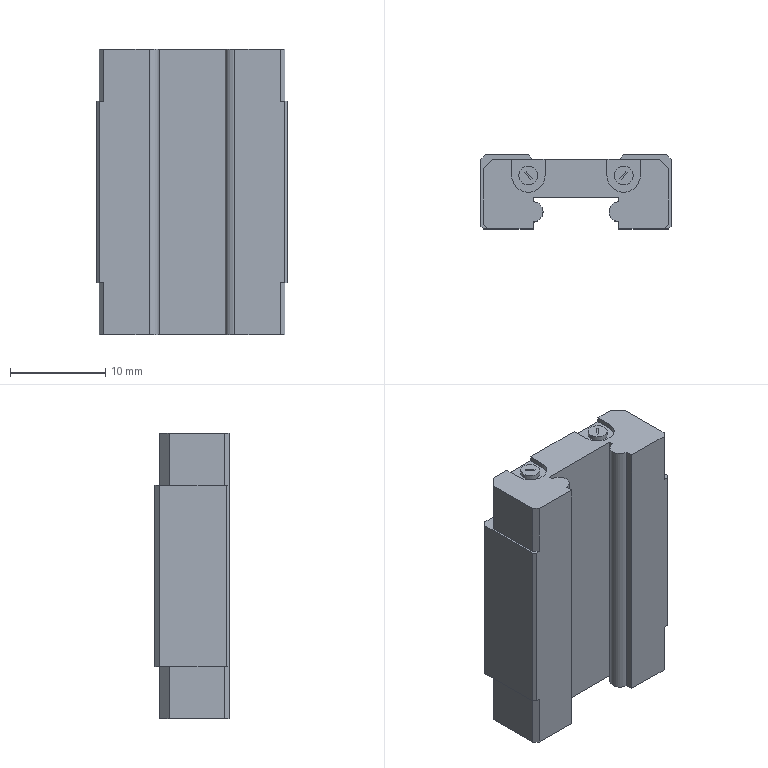Part | STEP file | SEBZ10-552 | 1 solid | 111 faces | box 20 x 7.8 x 30 mm | volume 3537 mm3 | plane 72 | cylinder 23 | cone 16 | commonest cylinder face diameters 2 x8 2.459 x8 3.5 x4 2.08 x3